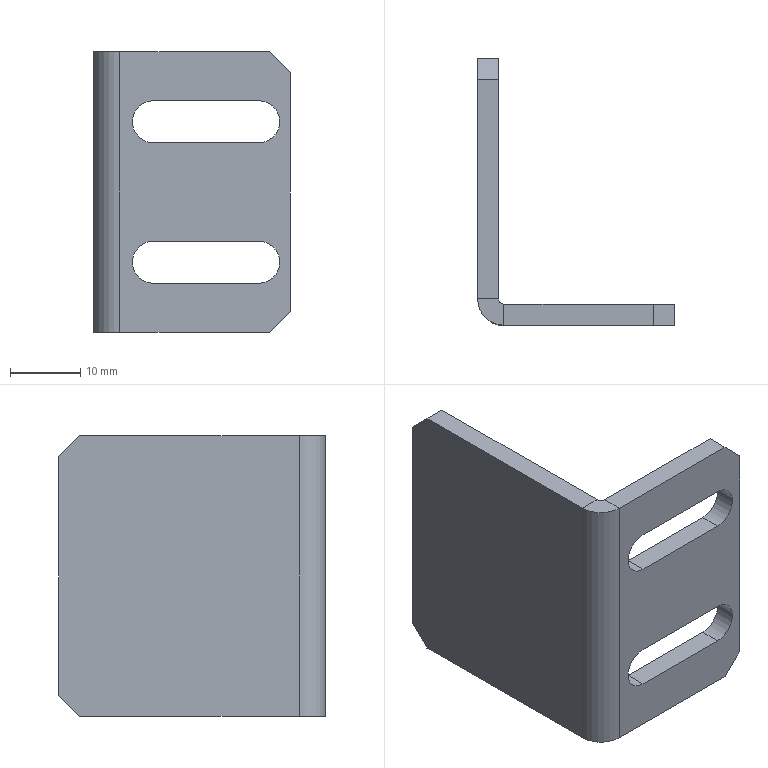Part | STEP file | 11-GYJJ-013-q11 | 1 solid | 26 faces | box 28 x 38 x 40 mm | volume 6681 mm3 | plane 20 | cylinder 6 | commonest cylinder face diameters 6 x4 1.473 x1 7.473 x1
STEP:
#1=CARTESIAN_POINT('',(0.7366,-35.,40.));
#2=VERTEX_POINT('',#1);
#3=CARTESIAN_POINT('',(0.7366,-38.,40.));
#4=VERTEX_POINT('',#3);
#5=CARTESIAN_POINT('',(0.7366,-35.,40.));
#6=DIRECTION('',(0.,-1.,0.));
#7=VECTOR('',#6,1000.);
#8=LINE('',#5,#7);
#9=EDGE_CURVE('',#2,#4,#8,.T.);
#10=ORIENTED_EDGE('',*,*,#9,.F.);
#11=CARTESIAN_POINT('',(0.,-34.263,40.));
#12=VERTEX_POINT('',#11);
#13=CARTESIAN_POINT('',(0.7366,-34.263,40.));
#14=DIRECTION('',(0.,0.,1.));
#15=DIRECTION('',(-1.,0.,0.));
#16=AXIS2_PLACEMENT_3D('',#13,#14,#15);
#17=CIRCLE('',#16,0.7366);
#18=EDGE_CURVE('',#12,#2,#17,.T.);
#19=ORIENTED_EDGE('',*,*,#18,.F.);
#20=CARTESIAN_POINT('',(-3.,-34.263,40.));
#21=VERTEX_POINT('',#20);
#22=CARTESIAN_POINT('',(-3.,-34.263,40.));
#23=DIRECTION('',(1.,0.,0.));
#24=VECTOR('',#23,1000.);
#25=LINE('',#22,#24);
#26=EDGE_CURVE('',#21,#12,#25,.T.);
#27=ORIENTED_EDGE('',*,*,#26,.F.);
#28=CARTESIAN_POINT('',(0.7366,-34.263,40.));
#29=DIRECTION('',(0.,0.,1.));
#30=DIRECTION('',(1.,0.,0.));
#31=AXIS2_PLACEMENT_3D('',#28,#29,#30);
#32=CIRCLE('',#31,3.737);
#33=EDGE_CURVE('',#21,#4,#32,.T.);
#34=ORIENTED_EDGE('',*,*,#33,.T.);
#35=EDGE_LOOP('',(#10,#19,#27,#34));
#36=FACE_OUTER_BOUND('',#35,.T.);
#37=CARTESIAN_POINT('',(0.7366,-35.,40.));
#38=DIRECTION('',(0.,0.,1.));
#39=DIRECTION('',(1.,0.,0.));
#40=AXIS2_PLACEMENT_3D('',#37,#38,#39);
#41=PLANE('',#40);
#42=ADVANCED_FACE('',(#36),#41,.T.);
#43=CARTESIAN_POINT('',(22.,-38.,40.));
#44=VERTEX_POINT('',#43);
#45=CARTESIAN_POINT('',(0.,-38.,40.));
#46=DIRECTION('',(1.,0.,0.));
#47=VECTOR('',#46,1000.);
#48=LINE('',#45,#47);
#49=EDGE_CURVE('',#4,#44,#48,.T.);
#50=ORIENTED_EDGE('',*,*,#49,.T.);
#51=CARTESIAN_POINT('',(22.,-35.,40.));
#52=VERTEX_POINT('',#51);
#53=CARTESIAN_POINT('',(22.,-34.263,40.));
#54=DIRECTION('',(0.,1.,0.));
#55=VECTOR('',#54,1000.);
#56=LINE('',#53,#55);
#57=EDGE_CURVE('',#44,#52,#56,.T.);
#58=ORIENTED_EDGE('',*,*,#57,.T.);
#59=CARTESIAN_POINT('',(0.,-35.,40.));
#60=DIRECTION('',(1.,0.,0.));
#61=VECTOR('',#60,1000.);
#62=LINE('',#59,#61);
#63=EDGE_CURVE('',#2,#52,#62,.T.);
#64=ORIENTED_EDGE('',*,*,#63,.F.);
#65=ORIENTED_EDGE('',*,*,#9,.T.);
#66=EDGE_LOOP('',(#50,#58,#64,#65));
#67=FACE_OUTER_BOUND('',#66,.T.);
#68=CARTESIAN_POINT('',(-3.,-34.263,40.));
#69=DIRECTION('',(0.,0.,1.));
#70=DIRECTION('',(1.,0.,0.));
#71=AXIS2_PLACEMENT_3D('',#68,#69,#70);
#72=PLANE('',#71);
#73=ADVANCED_FACE('',(#67),#72,.T.);
#74=CARTESIAN_POINT('',(0.,-34.263,0.));
#75=VERTEX_POINT('',#74);
#76=CARTESIAN_POINT('',(-3.,-34.263,0.));
#77=VERTEX_POINT('',#76);
#78=CARTESIAN_POINT('',(0.,-34.263,0.));
#79=DIRECTION('',(-1.,0.,0.));
#80=VECTOR('',#79,1000.);
#81=LINE('',#78,#80);
#82=EDGE_CURVE('',#75,#77,#81,.T.);
#83=ORIENTED_EDGE('',*,*,#82,.F.);
#84=CARTESIAN_POINT('',(0.7366,-35.,0.));
#85=VERTEX_POINT('',#84);
#86=CARTESIAN_POINT('',(0.7366,-34.263,0.));
#87=DIRECTION('',(0.,0.,1.));
#88=DIRECTION('',(-1.,0.,0.));
#89=AXIS2_PLACEMENT_3D('',#86,#87,#88);
#90=CIRCLE('',#89,0.7366);
#91=EDGE_CURVE('',#75,#85,#90,.T.);
#92=ORIENTED_EDGE('',*,*,#91,.T.);
#93=CARTESIAN_POINT('',(0.7366,-38.,0.));
#94=VERTEX_POINT('',#93);
#95=CARTESIAN_POINT('',(0.7366,-38.,0.));
#96=DIRECTION('',(0.,1.,0.));
#97=VECTOR('',#96,1000.);
#98=LINE('',#95,#97);
#99=EDGE_CURVE('',#94,#85,#98,.T.);
#100=ORIENTED_EDGE('',*,*,#99,.F.);
#101=CARTESIAN_POINT('',(0.7366,-34.263,0.));
#102=DIRECTION('',(0.,0.,1.));
#103=DIRECTION('',(1.,0.,0.));
#104=AXIS2_PLACEMENT_3D('',#101,#102,#103);
#105=CIRCLE('',#104,3.737);
#106=EDGE_CURVE('',#77,#94,#105,.T.);
#107=ORIENTED_EDGE('',*,*,#106,.F.);
#108=EDGE_LOOP('',(#83,#92,#100,#107));
#109=FACE_OUTER_BOUND('',#108,.T.);
#110=CARTESIAN_POINT('',(0.,-34.263,0.));
#111=DIRECTION('',(0.,0.,-1.));
#112=DIRECTION('',(-1.,0.,0.));
#113=AXIS2_PLACEMENT_3D('',#110,#111,#112);
#114=PLANE('',#113);
#115=ADVANCED_FACE('',(#109),#114,.T.);
#116=CARTESIAN_POINT('',(-3.,-3.,0.));
#117=VERTEX_POINT('',#116);
#118=CARTESIAN_POINT('',(-3.,0.,0.));
#119=DIRECTION('',(0.,-1.,0.));
#120=VECTOR('',#119,1000.);
#121=LINE('',#118,#120);
#122=EDGE_CURVE('',#117,#77,#121,.T.);
#123=ORIENTED_EDGE('',*,*,#122,.F.);
#124=CARTESIAN_POINT('',(0.,-3.,0.));
#125=VERTEX_POINT('',#124);
#126=CARTESIAN_POINT('',(0.7366,-3.,0.));
#127=DIRECTION('',(1.,0.,0.));
#128=VECTOR('',#127,1000.);
#129=LINE('',#126,#128);
#130=EDGE_CURVE('',#117,#125,#129,.T.);
#131=ORIENTED_EDGE('',*,*,#130,.T.);
#132=CARTESIAN_POINT('',(0.,0.,0.));
#133=DIRECTION('',(0.,-1.,0.));
#134=VECTOR('',#133,1000.);
#135=LINE('',#132,#134);
#136=EDGE_CURVE('',#125,#75,#135,.T.);
#137=ORIENTED_EDGE('',*,*,#136,.T.);
#138=ORIENTED_EDGE('',*,*,#82,.T.);
#139=EDGE_LOOP('',(#123,#131,#137,#138));
#140=FACE_OUTER_BOUND('',#139,.T.);
#141=CARTESIAN_POINT('',(0.7366,-38.,0.));
#142=DIRECTION('',(0.,0.,-1.));
#143=DIRECTION('',(-1.,0.,0.));
#144=AXIS2_PLACEMENT_3D('',#141,#142,#143);
#145=PLANE('',#144);
#146=ADVANCED_FACE('',(#140),#145,.T.);
#147=CARTESIAN_POINT('',(20.5,-38.,7.));
#148=VERTEX_POINT('',#147);
#149=CARTESIAN_POINT('',(5.5,-38.,7.));
#150=VERTEX_POINT('',#149);
#151=CARTESIAN_POINT('',(5.5,-38.,7.));
#152=DIRECTION('',(-1.,0.,0.));
#153=VECTOR('',#152,1000.);
#154=LINE('',#151,#153);
#155=EDGE_CURVE('',#148,#150,#154,.T.);
#156=ORIENTED_EDGE('',*,*,#155,.T.);
#157=CARTESIAN_POINT('',(5.5,-38.,13.));
#158=VERTEX_POINT('',#157);
#159=CARTESIAN_POINT('',(5.5,-38.,10.));
#160=DIRECTION('',(0.,1.,0.));
#161=DIRECTION('',(0.,0.,1.));
#162=AXIS2_PLACEMENT_3D('',#159,#160,#161);
#163=CIRCLE('',#162,3.);
#164=EDGE_CURVE('',#150,#158,#163,.T.);
#165=ORIENTED_EDGE('',*,*,#164,.T.);
#166=CARTESIAN_POINT('',(20.5,-38.,13.));
#167=VERTEX_POINT('',#166);
#168=CARTESIAN_POINT('',(5.5,-38.,13.));
#169=DIRECTION('',(1.,0.,0.));
#170=VECTOR('',#169,1000.);
#171=LINE('',#168,#170);
#172=EDGE_CURVE('',#158,#167,#171,.T.);
#173=ORIENTED_EDGE('',*,*,#172,.T.);
#174=CARTESIAN_POINT('',(20.5,-38.,10.));
#175=DIRECTION('',(0.,1.,0.));
#176=DIRECTION('',(0.,0.,1.));
#177=AXIS2_PLACEMENT_3D('',#174,#175,#176);
#178=CIRCLE('',#177,3.);
#179=EDGE_CURVE('',#167,#148,#178,.T.);
#180=ORIENTED_EDGE('',*,*,#179,.T.);
#181=EDGE_LOOP('',(#156,#165,#173,#180));
#182=FACE_BOUND('',#181,.T.);
#183=CARTESIAN_POINT('',(5.5,-38.,33.));
#184=VERTEX_POINT('',#183);
#185=CARTESIAN_POINT('',(20.5,-38.,33.));
#186=VERTEX_POINT('',#185);
#187=CARTESIAN_POINT('',(20.5,-38.,33.));
#188=DIRECTION('',(1.,0.,0.));
#189=VECTOR('',#188,1000.);
#190=LINE('',#187,#189);
#191=EDGE_CURVE('',#184,#186,#190,.T.);
#192=ORIENTED_EDGE('',*,*,#191,.T.);
#193=CARTESIAN_POINT('',(20.5,-38.,27.));
#194=VERTEX_POINT('',#193);
#195=CARTESIAN_POINT('',(20.5,-38.,30.));
#196=DIRECTION('',(0.,1.,0.));
#197=DIRECTION('',(0.,0.,1.));
#198=AXIS2_PLACEMENT_3D('',#195,#196,#197);
#199=CIRCLE('',#198,3.);
#200=EDGE_CURVE('',#186,#194,#199,.T.);
#201=ORIENTED_EDGE('',*,*,#200,.T.);
#202=CARTESIAN_POINT('',(5.5,-38.,27.));
#203=VERTEX_POINT('',#202);
#204=CARTESIAN_POINT('',(20.5,-38.,27.));
#205=DIRECTION('',(-1.,0.,0.));
#206=VECTOR('',#205,1000.);
#207=LINE('',#204,#206);
#208=EDGE_CURVE('',#194,#203,#207,.T.);
#209=ORIENTED_EDGE('',*,*,#208,.T.);
#210=CARTESIAN_POINT('',(5.5,-38.,30.));
#211=DIRECTION('',(0.,1.,0.));
#212=DIRECTION('',(0.,0.,1.));
#213=AXIS2_PLACEMENT_3D('',#210,#211,#212);
#214=CIRCLE('',#213,3.);
#215=EDGE_CURVE('',#203,#184,#214,.T.);
#216=ORIENTED_EDGE('',*,*,#215,.T.);
#217=EDGE_LOOP('',(#192,#201,#209,#216));
#218=FACE_BOUND('',#217,.T.);
#219=CARTESIAN_POINT('',(25.,-38.,37.));
#220=VERTEX_POINT('',#219);
#221=CARTESIAN_POINT('',(25.,-38.,3.));
#222=VERTEX_POINT('',#221);
#223=CARTESIAN_POINT('',(25.,-38.,40.));
#224=DIRECTION('',(0.,0.,-1.));
#225=VECTOR('',#224,1000.);
#226=LINE('',#223,#225);
#227=EDGE_CURVE('',#220,#222,#226,.T.);
#228=ORIENTED_EDGE('',*,*,#227,.F.);
#229=CARTESIAN_POINT('',(25.,-38.,37.));
#230=DIRECTION('',(-0.7071,0.,0.7071));
#231=VECTOR('',#230,1000.);
#232=LINE('',#229,#231);
#233=EDGE_CURVE('',#220,#44,#232,.T.);
#234=ORIENTED_EDGE('',*,*,#233,.T.);
#235=ORIENTED_EDGE('',*,*,#49,.F.);
#236=CARTESIAN_POINT('',(0.7366,-38.,40.));
#237=DIRECTION('',(0.,0.,-1.));
#238=VECTOR('',#237,1000.);
#239=LINE('',#236,#238);
#240=EDGE_CURVE('',#4,#94,#239,.T.);
#241=ORIENTED_EDGE('',*,*,#240,.T.);
#242=CARTESIAN_POINT('',(22.,-38.,0.));
#243=VERTEX_POINT('',#242);
#244=CARTESIAN_POINT('',(0.,-38.,0.));
#245=DIRECTION('',(1.,0.,0.));
#246=VECTOR('',#245,1000.);
#247=LINE('',#244,#246);
#248=EDGE_CURVE('',#94,#243,#247,.T.);
#249=ORIENTED_EDGE('',*,*,#248,.T.);
#250=CARTESIAN_POINT('',(22.,-38.,0.));
#251=DIRECTION('',(0.7071,0.,0.7071));
#252=VECTOR('',#251,1000.);
#253=LINE('',#250,#252);
#254=EDGE_CURVE('',#243,#222,#253,.T.);
#255=ORIENTED_EDGE('',*,*,#254,.T.);
#256=EDGE_LOOP('',(#228,#234,#235,#241,#249,#255));
#257=FACE_OUTER_BOUND('',#256,.T.);
#258=CARTESIAN_POINT('',(0.,-38.,40.));
#259=DIRECTION('',(0.,1.,0.));
#260=DIRECTION('',(0.,0.,1.));
#261=AXIS2_PLACEMENT_3D('',#258,#259,#260);
#262=PLANE('',#261);
#263=ADVANCED_FACE('',(#182,#218,#257),#262,.F.);
#264=CARTESIAN_POINT('',(25.,-35.,37.));
#265=VERTEX_POINT('',#264);
#266=CARTESIAN_POINT('',(25.,-35.,3.));
#267=VERTEX_POINT('',#266);
#268=CARTESIAN_POINT('',(25.,-35.,40.));
#269=DIRECTION('',(0.,0.,-1.));
#270=VECTOR('',#269,1000.);
#271=LINE('',#268,#270);
#272=EDGE_CURVE('',#265,#267,#271,.T.);
#273=ORIENTED_EDGE('',*,*,#272,.F.);
#274=CARTESIAN_POINT('',(25.,-35.,37.));
#275=DIRECTION('',(0.,-1.,0.));
#276=VECTOR('',#275,1000.);
#277=LINE('',#274,#276);
#278=EDGE_CURVE('',#265,#220,#277,.T.);
#279=ORIENTED_EDGE('',*,*,#278,.T.);
#280=ORIENTED_EDGE('',*,*,#227,.T.);
#281=CARTESIAN_POINT('',(25.,-35.,3.));
#282=DIRECTION('',(0.,1.,0.));
#283=VECTOR('',#282,1000.);
#284=LINE('',#281,#283);
#285=EDGE_CURVE('',#222,#267,#284,.T.);
#286=ORIENTED_EDGE('',*,*,#285,.T.);
#287=EDGE_LOOP('',(#273,#279,#280,#286));
#288=FACE_OUTER_BOUND('',#287,.T.);
#289=CARTESIAN_POINT('',(25.,-35.,40.));
#290=DIRECTION('',(1.,0.,0.));
#291=DIRECTION('',(0.,0.,-1.));
#292=AXIS2_PLACEMENT_3D('',#289,#290,#291);
#293=PLANE('',#292);
#294=ADVANCED_FACE('',(#288),#293,.T.);
#295=CARTESIAN_POINT('',(5.5,-35.,7.));
#296=VERTEX_POINT('',#295);
#297=CARTESIAN_POINT('',(5.5,-35.,13.));
#298=VERTEX_POINT('',#297);
#299=CARTESIAN_POINT('',(5.5,-35.,10.));
#300=DIRECTION('',(0.,1.,0.));
#301=DIRECTION('',(0.,0.,1.));
#302=AXIS2_PLACEMENT_3D('',#299,#300,#301);
#303=CIRCLE('',#302,3.);
#304=EDGE_CURVE('',#296,#298,#303,.T.);
#305=ORIENTED_EDGE('',*,*,#304,.F.);
#306=CARTESIAN_POINT('',(20.5,-35.,7.));
#307=VERTEX_POINT('',#306);
#308=CARTESIAN_POINT('',(5.5,-35.,7.));
#309=DIRECTION('',(-1.,0.,0.));
#310=VECTOR('',#309,1000.);
#311=LINE('',#308,#310);
#312=EDGE_CURVE('',#307,#296,#311,.T.);
#313=ORIENTED_EDGE('',*,*,#312,.F.);
#314=CARTESIAN_POINT('',(20.5,-35.,13.));
#315=VERTEX_POINT('',#314);
#316=CARTESIAN_POINT('',(20.5,-35.,10.));
#317=DIRECTION('',(0.,1.,0.));
#318=DIRECTION('',(0.,0.,1.));
#319=AXIS2_PLACEMENT_3D('',#316,#317,#318);
#320=CIRCLE('',#319,3.);
#321=EDGE_CURVE('',#315,#307,#320,.T.);
#322=ORIENTED_EDGE('',*,*,#321,.F.);
#323=CARTESIAN_POINT('',(5.5,-35.,13.));
#324=DIRECTION('',(1.,0.,0.));
#325=VECTOR('',#324,1000.);
#326=LINE('',#323,#325);
#327=EDGE_CURVE('',#298,#315,#326,.T.);
#328=ORIENTED_EDGE('',*,*,#327,.F.);
#329=EDGE_LOOP('',(#305,#313,#322,#328));
#330=FACE_BOUND('',#329,.T.);
#331=CARTESIAN_POINT('',(20.5,-35.,33.));
#332=VERTEX_POINT('',#331);
#333=CARTESIAN_POINT('',(20.5,-35.,27.));
#334=VERTEX_POINT('',#333);
#335=CARTESIAN_POINT('',(20.5,-35.,30.));
#336=DIRECTION('',(0.,1.,0.));
#337=DIRECTION('',(0.,0.,1.));
#338=AXIS2_PLACEMENT_3D('',#335,#336,#337);
#339=CIRCLE('',#338,3.);
#340=EDGE_CURVE('',#332,#334,#339,.T.);
#341=ORIENTED_EDGE('',*,*,#340,.F.);
#342=CARTESIAN_POINT('',(5.5,-35.,33.));
#343=VERTEX_POINT('',#342);
#344=CARTESIAN_POINT('',(20.5,-35.,33.));
#345=DIRECTION('',(1.,0.,0.));
#346=VECTOR('',#345,1000.);
#347=LINE('',#344,#346);
#348=EDGE_CURVE('',#343,#332,#347,.T.);
#349=ORIENTED_EDGE('',*,*,#348,.F.);
#350=CARTESIAN_POINT('',(5.5,-35.,27.));
#351=VERTEX_POINT('',#350);
#352=CARTESIAN_POINT('',(5.5,-35.,30.));
#353=DIRECTION('',(0.,1.,0.));
#354=DIRECTION('',(0.,0.,1.));
#355=AXIS2_PLACEMENT_3D('',#352,#353,#354);
#356=CIRCLE('',#355,3.);
#357=EDGE_CURVE('',#351,#343,#356,.T.);
#358=ORIENTED_EDGE('',*,*,#357,.F.);
#359=CARTESIAN_POINT('',(20.5,-35.,27.));
#360=DIRECTION('',(-1.,0.,0.));
#361=VECTOR('',#360,1000.);
#362=LINE('',#359,#361);
#363=EDGE_CURVE('',#334,#351,#362,.T.);
#364=ORIENTED_EDGE('',*,*,#363,.F.);
#365=EDGE_LOOP('',(#341,#349,#358,#364));
#366=FACE_BOUND('',#365,.T.);
#367=ORIENTED_EDGE('',*,*,#63,.T.);
#368=CARTESIAN_POINT('',(11.,-35.,51.));
#369=DIRECTION('',(0.7071,0.,-0.7071));
#370=VECTOR('',#369,1000.);
#371=LINE('',#368,#370);
#372=EDGE_CURVE('',#52,#265,#371,.T.);
#373=ORIENTED_EDGE('',*,*,#372,.T.);
#374=ORIENTED_EDGE('',*,*,#272,.T.);
#375=CARTESIAN_POINT('',(22.,-35.,0.));
#376=VERTEX_POINT('',#375);
#377=CARTESIAN_POINT('',(31.,-35.,9.));
#378=DIRECTION('',(-0.7071,0.,-0.7071));
#379=VECTOR('',#378,1000.);
#380=LINE('',#377,#379);
#381=EDGE_CURVE('',#267,#376,#380,.T.);
#382=ORIENTED_EDGE('',*,*,#381,.T.);
#383=CARTESIAN_POINT('',(0.,-35.,0.));
#384=DIRECTION('',(1.,0.,0.));
#385=VECTOR('',#384,1000.);
#386=LINE('',#383,#385);
#387=EDGE_CURVE('',#85,#376,#386,.T.);
#388=ORIENTED_EDGE('',*,*,#387,.F.);
#389=CARTESIAN_POINT('',(0.7366,-35.,40.));
#390=DIRECTION('',(0.,0.,-1.));
#391=VECTOR('',#390,1000.);
#392=LINE('',#389,#391);
#393=EDGE_CURVE('',#2,#85,#392,.T.);
#394=ORIENTED_EDGE('',*,*,#393,.F.);
#395=EDGE_LOOP('',(#367,#373,#374,#382,#388,#394));
#396=FACE_OUTER_BOUND('',#395,.T.);
#397=CARTESIAN_POINT('',(0.,-35.,40.));
#398=DIRECTION('',(0.,1.,0.));
#399=DIRECTION('',(0.,0.,1.));
#400=AXIS2_PLACEMENT_3D('',#397,#398,#399);
#401=PLANE('',#400);
#402=ADVANCED_FACE('',(#330,#366,#396),#401,.T.);
#403=ORIENTED_EDGE('',*,*,#91,.F.);
#404=CARTESIAN_POINT('',(0.,-34.263,40.));
#405=DIRECTION('',(0.,0.,-1.));
#406=VECTOR('',#405,1000.);
#407=LINE('',#404,#406);
#408=EDGE_CURVE('',#12,#75,#407,.T.);
#409=ORIENTED_EDGE('',*,*,#408,.F.);
#410=ORIENTED_EDGE('',*,*,#18,.T.);
#411=ORIENTED_EDGE('',*,*,#393,.T.);
#412=EDGE_LOOP('',(#403,#409,#410,#411));
#413=FACE_OUTER_BOUND('',#412,.T.);
#414=CARTESIAN_POINT('',(0.7366,-34.263,40.));
#415=DIRECTION('',(0.,0.,-1.));
#416=DIRECTION('',(-1.,0.,0.));
#417=AXIS2_PLACEMENT_3D('',#414,#415,#416);
#418=CYLINDRICAL_SURFACE('',#417,0.7366);
#419=ADVANCED_FACE('',(#413),#418,.F.);
#420=CARTESIAN_POINT('',(0.,0.,37.));
#421=VERTEX_POINT('',#420);
#422=CARTESIAN_POINT('',(0.,0.,3.));
#423=VERTEX_POINT('',#422);
#424=CARTESIAN_POINT('',(0.,0.,40.));
#425=DIRECTION('',(0.,0.,-1.));
#426=VECTOR('',#425,1000.);
#427=LINE('',#424,#426);
#428=EDGE_CURVE('',#421,#423,#427,.T.);
#429=ORIENTED_EDGE('',*,*,#428,.F.);
#430=CARTESIAN_POINT('',(0.,-3.,40.));
#431=VERTEX_POINT('',#430);
#432=CARTESIAN_POINT('',(0.,-1.5,38.5));
#433=DIRECTION('',(0.,-0.7071,0.7071));
#434=VECTOR('',#433,1000.);
#435=LINE('',#432,#434);
#436=EDGE_CURVE('',#421,#431,#435,.T.);
#437=ORIENTED_EDGE('',*,*,#436,.T.);
#438=CARTESIAN_POINT('',(0.,0.,40.));
#439=DIRECTION('',(0.,-1.,0.));
#440=VECTOR('',#439,1000.);
#441=LINE('',#438,#440);
#442=EDGE_CURVE('',#431,#12,#441,.T.);
#443=ORIENTED_EDGE('',*,*,#442,.T.);
#444=ORIENTED_EDGE('',*,*,#408,.T.);
#445=ORIENTED_EDGE('',*,*,#136,.F.);
#446=CARTESIAN_POINT('',(0.,18.5,21.5));
#447=DIRECTION('',(0.,0.7071,0.7071));
#448=VECTOR('',#447,1000.);
#449=LINE('',#446,#448);
#450=EDGE_CURVE('',#125,#423,#449,.T.);
#451=ORIENTED_EDGE('',*,*,#450,.T.);
#452=EDGE_LOOP('',(#429,#437,#443,#444,#445,#451));
#453=FACE_OUTER_BOUND('',#452,.T.);
#454=CARTESIAN_POINT('',(0.,0.,40.));
#455=DIRECTION('',(1.,0.,0.));
#456=DIRECTION('',(0.,1.,0.));
#457=AXIS2_PLACEMENT_3D('',#454,#455,#456);
#458=PLANE('',#457);
#459=ADVANCED_FACE('',(#453),#458,.T.);
#460=CARTESIAN_POINT('',(-3.,0.,37.));
#461=VERTEX_POINT('',#460);
#462=CARTESIAN_POINT('',(-3.,0.,3.));
#463=VERTEX_POINT('',#462);
#464=CARTESIAN_POINT('',(-3.,0.,40.));
#465=DIRECTION('',(0.,0.,-1.));
#466=VECTOR('',#465,1000.);
#467=LINE('',#464,#466);
#468=EDGE_CURVE('',#461,#463,#467,.T.);
#469=ORIENTED_EDGE('',*,*,#468,.F.);
#470=CARTESIAN_POINT('',(0.,0.,37.));
#471=DIRECTION('',(1.,0.,0.));
#472=VECTOR('',#471,1000.);
#473=LINE('',#470,#472);
#474=EDGE_CURVE('',#461,#421,#473,.T.);
#475=ORIENTED_EDGE('',*,*,#474,.T.);
#476=ORIENTED_EDGE('',*,*,#428,.T.);
#477=CARTESIAN_POINT('',(-3.,0.,3.));
#478=DIRECTION('',(-1.,0.,0.));
#479=VECTOR('',#478,1000.);
#480=LINE('',#477,#479);
#481=EDGE_CURVE('',#423,#463,#480,.T.);
#482=ORIENTED_EDGE('',*,*,#481,.T.);
#483=EDGE_LOOP('',(#469,#475,#476,#482));
#484=FACE_OUTER_BOUND('',#483,.T.);
#485=CARTESIAN_POINT('',(-3.,0.,40.));
#486=DIRECTION('',(0.,1.,0.));
#487=DIRECTION('',(-1.,0.,0.));
#488=AXIS2_PLACEMENT_3D('',#485,#486,#487);
#489=PLANE('',#488);
#490=ADVANCED_FACE('',(#484),#489,.T.);
#491=CARTESIAN_POINT('',(-3.,-3.,40.));
#492=VERTEX_POINT('',#491);
#493=CARTESIAN_POINT('',(-3.,0.,40.));
#494=DIRECTION('',(0.,-1.,0.));
#495=VECTOR('',#494,1000.);
#496=LINE('',#493,#495);
#497=EDGE_CURVE('',#492,#21,#496,.T.);
#498=ORIENTED_EDGE('',*,*,#497,.F.);
#499=CARTESIAN_POINT('',(-3.,0.,37.));
#500=DIRECTION('',(0.,0.7071,-0.7071));
#501=VECTOR('',#500,1000.);
#502=LINE('',#499,#501);
#503=EDGE_CURVE('',#492,#461,#502,.T.);
#504=ORIENTED_EDGE('',*,*,#503,.T.);
#505=ORIENTED_EDGE('',*,*,#468,.T.);
#506=CARTESIAN_POINT('',(-3.,-3.,0.));
#507=DIRECTION('',(0.,-0.7071,-0.7071));
#508=VECTOR('',#507,1000.);
#509=LINE('',#506,#508);
#510=EDGE_CURVE('',#463,#117,#509,.T.);
#511=ORIENTED_EDGE('',*,*,#510,.T.);
#512=ORIENTED_EDGE('',*,*,#122,.T.);
#513=CARTESIAN_POINT('',(-3.,-34.263,40.));
#514=DIRECTION('',(0.,0.,-1.));
#515=VECTOR('',#514,1000.);
#516=LINE('',#513,#515);
#517=EDGE_CURVE('',#21,#77,#516,.T.);
#518=ORIENTED_EDGE('',*,*,#517,.F.);
#519=EDGE_LOOP('',(#498,#504,#505,#511,#512,#518));
#520=FACE_OUTER_BOUND('',#519,.T.);
#521=CARTESIAN_POINT('',(-3.,0.,40.));
#522=DIRECTION('',(1.,0.,0.));
#523=DIRECTION('',(0.,1.,0.));
#524=AXIS2_PLACEMENT_3D('',#521,#522,#523);
#525=PLANE('',#524);
#526=ADVANCED_FACE('',(#520),#525,.F.);
#527=ORIENTED_EDGE('',*,*,#106,.T.);
#528=ORIENTED_EDGE('',*,*,#240,.F.);
#529=ORIENTED_EDGE('',*,*,#33,.F.);
#530=ORIENTED_EDGE('',*,*,#517,.T.);
#531=EDGE_LOOP('',(#527,#528,#529,#530));
#532=FACE_OUTER_BOUND('',#531,.T.);
#533=CARTESIAN_POINT('',(0.7366,-34.263,40.));
#534=DIRECTION('',(0.,0.,-1.));
#535=DIRECTION('',(-1.,0.,0.));
#536=AXIS2_PLACEMENT_3D('',#533,#534,#535);
#537=CYLINDRICAL_SURFACE('',#536,3.737);
#538=ADVANCED_FACE('',(#532),#537,.T.);
#539=ORIENTED_EDGE('',*,*,#442,.F.);
#540=CARTESIAN_POINT('',(-3.,-3.,40.));
#541=DIRECTION('',(-1.,0.,0.));
#542=VECTOR('',#541,1000.);
#543=LINE('',#540,#542);
#544=EDGE_CURVE('',#431,#492,#543,.T.);
#545=ORIENTED_EDGE('',*,*,#544,.T.);
#546=ORIENTED_EDGE('',*,*,#497,.T.);
#547=ORIENTED_EDGE('',*,*,#26,.T.);
#548=EDGE_LOOP('',(#539,#545,#546,#547));
#549=FACE_OUTER_BOUND('',#548,.T.);
#550=CARTESIAN_POINT('',(0.7366,-34.263,40.));
#551=DIRECTION('',(0.,0.,-1.));
#552=DIRECTION('',(-1.,0.,0.));
#553=AXIS2_PLACEMENT_3D('',#550,#551,#552);
#554=PLANE('',#553);
#555=ADVANCED_FACE('',(#549),#554,.F.);
#556=ORIENTED_EDGE('',*,*,#387,.T.);
#557=CARTESIAN_POINT('',(22.,-34.263,0.));
#558=DIRECTION('',(0.,-1.,0.));
#559=VECTOR('',#558,1000.);
#560=LINE('',#557,#559);
#561=EDGE_CURVE('',#376,#243,#560,.T.);
#562=ORIENTED_EDGE('',*,*,#561,.T.);
#563=ORIENTED_EDGE('',*,*,#248,.F.);
#564=ORIENTED_EDGE('',*,*,#99,.T.);
#565=EDGE_LOOP('',(#556,#562,#563,#564));
#566=FACE_OUTER_BOUND('',#565,.T.);
#567=CARTESIAN_POINT('',(0.7366,-34.263,0.));
#568=DIRECTION('',(0.,0.,-1.));
#569=DIRECTION('',(-1.,0.,0.));
#570=AXIS2_PLACEMENT_3D('',#567,#568,#569);
#571=PLANE('',#570);
#572=ADVANCED_FACE('',(#566),#571,.T.);
#573=ORIENTED_EDGE('',*,*,#372,.F.);
#574=ORIENTED_EDGE('',*,*,#57,.F.);
#575=ORIENTED_EDGE('',*,*,#233,.F.);
#576=ORIENTED_EDGE('',*,*,#278,.F.);
#577=EDGE_LOOP('',(#573,#574,#575,#576));
#578=FACE_OUTER_BOUND('',#577,.T.);
#579=CARTESIAN_POINT('',(25.,-35.,37.));
#580=DIRECTION('',(-0.7071,0.,-0.7071));
#581=DIRECTION('',(0.,-1.,0.));
#582=AXIS2_PLACEMENT_3D('',#579,#580,#581);
#583=PLANE('',#582);
#584=ADVANCED_FACE('',(#578),#583,.F.);
#585=ORIENTED_EDGE('',*,*,#381,.F.);
#586=ORIENTED_EDGE('',*,*,#285,.F.);
#587=ORIENTED_EDGE('',*,*,#254,.F.);
#588=ORIENTED_EDGE('',*,*,#561,.F.);
#589=EDGE_LOOP('',(#585,#586,#587,#588));
#590=FACE_OUTER_BOUND('',#589,.T.);
#591=CARTESIAN_POINT('',(22.,-34.263,0.));
#592=DIRECTION('',(-0.7071,0.,0.7071));
#593=DIRECTION('',(0.,-1.,0.));
#594=AXIS2_PLACEMENT_3D('',#591,#592,#593);
#595=PLANE('',#594);
#596=ADVANCED_FACE('',(#590),#595,.F.);
#597=ORIENTED_EDGE('',*,*,#503,.F.);
#598=ORIENTED_EDGE('',*,*,#544,.F.);
#599=ORIENTED_EDGE('',*,*,#436,.F.);
#600=ORIENTED_EDGE('',*,*,#474,.F.);
#601=EDGE_LOOP('',(#597,#598,#599,#600));
#602=FACE_OUTER_BOUND('',#601,.T.);
#603=CARTESIAN_POINT('',(-3.,0.,37.));
#604=DIRECTION('',(0.,0.7071,0.7071));
#605=DIRECTION('',(-1.,0.,0.));
#606=AXIS2_PLACEMENT_3D('',#603,#604,#605);
#607=PLANE('',#606);
#608=ADVANCED_FACE('',(#602),#607,.T.);
#609=ORIENTED_EDGE('',*,*,#510,.F.);
#610=ORIENTED_EDGE('',*,*,#481,.F.);
#611=ORIENTED_EDGE('',*,*,#450,.F.);
#612=ORIENTED_EDGE('',*,*,#130,.F.);
#613=EDGE_LOOP('',(#609,#610,#611,#612));
#614=FACE_OUTER_BOUND('',#613,.T.);
#615=CARTESIAN_POINT('',(0.7366,-3.,0.));
#616=DIRECTION('',(0.,-0.7071,0.7071));
#617=DIRECTION('',(1.,0.,0.));
#618=AXIS2_PLACEMENT_3D('',#615,#616,#617);
#619=PLANE('',#618);
#620=ADVANCED_FACE('',(#614),#619,.F.);
#621=ORIENTED_EDGE('',*,*,#340,.T.);
#622=CARTESIAN_POINT('',(20.5,-38.,27.));
#623=DIRECTION('',(0.,1.,0.));
#624=VECTOR('',#623,1000.);
#625=LINE('',#622,#624);
#626=EDGE_CURVE('',#194,#334,#625,.T.);
#627=ORIENTED_EDGE('',*,*,#626,.F.);
#628=ORIENTED_EDGE('',*,*,#200,.F.);
#629=CARTESIAN_POINT('',(20.5,-38.,33.));
#630=DIRECTION('',(0.,1.,0.));
#631=VECTOR('',#630,1000.);
#632=LINE('',#629,#631);
#633=EDGE_CURVE('',#186,#332,#632,.T.);
#634=ORIENTED_EDGE('',*,*,#633,.T.);
#635=EDGE_LOOP('',(#621,#627,#628,#634));
#636=FACE_OUTER_BOUND('',#635,.T.);
#637=CARTESIAN_POINT('',(20.5,-38.,30.));
#638=DIRECTION('',(0.,1.,0.));
#639=DIRECTION('',(0.,0.,1.));
#640=AXIS2_PLACEMENT_3D('',#637,#638,#639);
#641=CYLINDRICAL_SURFACE('',#640,3.);
#642=ADVANCED_FACE('',(#636),#641,.F.);
#643=ORIENTED_EDGE('',*,*,#348,.T.);
#644=ORIENTED_EDGE('',*,*,#633,.F.);
#645=ORIENTED_EDGE('',*,*,#191,.F.);
#646=CARTESIAN_POINT('',(5.5,-38.,33.));
#647=DIRECTION('',(0.,1.,0.));
#648=VECTOR('',#647,1000.);
#649=LINE('',#646,#648);
#650=EDGE_CURVE('',#184,#343,#649,.T.);
#651=ORIENTED_EDGE('',*,*,#650,.T.);
#652=EDGE_LOOP('',(#643,#644,#645,#651));
#653=FACE_OUTER_BOUND('',#652,.T.);
#654=CARTESIAN_POINT('',(20.5,-38.,33.));
#655=DIRECTION('',(0.,0.,1.));
#656=DIRECTION('',(1.,0.,0.));
#657=AXIS2_PLACEMENT_3D('',#654,#655,#656);
#658=PLANE('',#657);
#659=ADVANCED_FACE('',(#653),#658,.F.);
#660=ORIENTED_EDGE('',*,*,#357,.T.);
#661=ORIENTED_EDGE('',*,*,#650,.F.);
#662=ORIENTED_EDGE('',*,*,#215,.F.);
#663=CARTESIAN_POINT('',(5.5,-38.,27.));
#664=DIRECTION('',(0.,1.,0.));
#665=VECTOR('',#664,1000.);
#666=LINE('',#663,#665);
#667=EDGE_CURVE('',#203,#351,#666,.T.);
#668=ORIENTED_EDGE('',*,*,#667,.T.);
#669=EDGE_LOOP('',(#660,#661,#662,#668));
#670=FACE_OUTER_BOUND('',#669,.T.);
#671=CARTESIAN_POINT('',(5.5,-38.,30.));
#672=DIRECTION('',(0.,1.,0.));
#673=DIRECTION('',(0.,0.,1.));
#674=AXIS2_PLACEMENT_3D('',#671,#672,#673);
#675=CYLINDRICAL_SURFACE('',#674,3.);
#676=ADVANCED_FACE('',(#670),#675,.F.);
#677=ORIENTED_EDGE('',*,*,#363,.T.);
#678=ORIENTED_EDGE('',*,*,#667,.F.);
#679=ORIENTED_EDGE('',*,*,#208,.F.);
#680=ORIENTED_EDGE('',*,*,#626,.T.);
#681=EDGE_LOOP('',(#677,#678,#679,#680));
#682=FACE_OUTER_BOUND('',#681,.T.);
#683=CARTESIAN_POINT('',(20.5,-38.,27.));
#684=DIRECTION('',(0.,0.,-1.));
#685=DIRECTION('',(-1.,0.,0.));
#686=AXIS2_PLACEMENT_3D('',#683,#684,#685);
#687=PLANE('',#686);
#688=ADVANCED_FACE('',(#682),#687,.F.);
#689=ORIENTED_EDGE('',*,*,#304,.T.);
#690=CARTESIAN_POINT('',(5.5,-38.,13.));
#691=DIRECTION('',(0.,1.,0.));
#692=VECTOR('',#691,1000.);
#693=LINE('',#690,#692);
#694=EDGE_CURVE('',#158,#298,#693,.T.);
#695=ORIENTED_EDGE('',*,*,#694,.F.);
#696=ORIENTED_EDGE('',*,*,#164,.F.);
#697=CARTESIAN_POINT('',(5.5,-38.,7.));
#698=DIRECTION('',(0.,1.,0.));
#699=VECTOR('',#698,1000.);
#700=LINE('',#697,#699);
#701=EDGE_CURVE('',#150,#296,#700,.T.);
#702=ORIENTED_EDGE('',*,*,#701,.T.);
#703=EDGE_LOOP('',(#689,#695,#696,#702));
#704=FACE_OUTER_BOUND('',#703,.T.);
#705=CARTESIAN_POINT('',(5.5,-38.,10.));
#706=DIRECTION('',(0.,1.,0.));
#707=DIRECTION('',(0.,0.,1.));
#708=AXIS2_PLACEMENT_3D('',#705,#706,#707);
#709=CYLINDRICAL_SURFACE('',#708,3.);
#710=ADVANCED_FACE('',(#704),#709,.F.);
#711=ORIENTED_EDGE('',*,*,#312,.T.);
#712=ORIENTED_EDGE('',*,*,#701,.F.);
#713=ORIENTED_EDGE('',*,*,#155,.F.);
#714=CARTESIAN_POINT('',(20.5,-38.,7.));
#715=DIRECTION('',(0.,1.,0.));
#716=VECTOR('',#715,1000.);
#717=LINE('',#714,#716);
#718=EDGE_CURVE('',#148,#307,#717,.T.);
#719=ORIENTED_EDGE('',*,*,#718,.T.);
#720=EDGE_LOOP('',(#711,#712,#713,#719));
#721=FACE_OUTER_BOUND('',#720,.T.);
#722=CARTESIAN_POINT('',(5.5,-38.,7.));
#723=DIRECTION('',(0.,0.,-1.));
#724=DIRECTION('',(-1.,0.,0.));
#725=AXIS2_PLACEMENT_3D('',#722,#723,#724);
#726=PLANE('',#725);
#727=ADVANCED_FACE('',(#721),#726,.F.);
#728=ORIENTED_EDGE('',*,*,#321,.T.);
#729=ORIENTED_EDGE('',*,*,#718,.F.);
#730=ORIENTED_EDGE('',*,*,#179,.F.);
#731=CARTESIAN_POINT('',(20.5,-38.,13.));
#732=DIRECTION('',(0.,1.,0.));
#733=VECTOR('',#732,1000.);
#734=LINE('',#731,#733);
#735=EDGE_CURVE('',#167,#315,#734,.T.);
#736=ORIENTED_EDGE('',*,*,#735,.T.);
#737=EDGE_LOOP('',(#728,#729,#730,#736));
#738=FACE_OUTER_BOUND('',#737,.T.);
#739=CARTESIAN_POINT('',(20.5,-38.,10.));
#740=DIRECTION('',(0.,1.,0.));
#741=DIRECTION('',(0.,0.,1.));
#742=AXIS2_PLACEMENT_3D('',#739,#740,#741);
#743=CYLINDRICAL_SURFACE('',#742,3.);
#744=ADVANCED_FACE('',(#738),#743,.F.);
#745=ORIENTED_EDGE('',*,*,#327,.T.);
#746=ORIENTED_EDGE('',*,*,#735,.F.);
#747=ORIENTED_EDGE('',*,*,#172,.F.);
#748=ORIENTED_EDGE('',*,*,#694,.T.);
#749=EDGE_LOOP('',(#745,#746,#747,#748));
#750=FACE_OUTER_BOUND('',#749,.T.);
#751=CARTESIAN_POINT('',(5.5,-38.,13.));
#752=DIRECTION('',(0.,0.,1.));
#753=DIRECTION('',(1.,0.,0.));
#754=AXIS2_PLACEMENT_3D('',#751,#752,#753);
#755=PLANE('',#754);
#756=ADVANCED_FACE('',(#750),#755,.F.);
#757=CLOSED_SHELL('',(#42,#73,#115,#146,#263,#294,#402,#419,#459,#490,#526,#538,#555,#572,#584,#596,#608,#620,#642,#659,#676,#688,#710,#727,#744,#756));
#758=MANIFOLD_SOLID_BREP('',#757);
#759=CARTESIAN_POINT('',(0.,0.,0.));
#760=DIRECTION('',(0.,0.,1.));
#761=DIRECTION('',(1.,0.,0.));
#762=AXIS2_PLACEMENT_3D('',#759,#760,#761);
#763=(LENGTH_UNIT()NAMED_UNIT(*)SI_UNIT(.MILLI.,.METRE.));
#764=UNCERTAINTY_MEASURE_WITH_UNIT(LENGTH_MEASURE(0.00001),#763,'','');
#765=(NAMED_UNIT(*)PLANE_ANGLE_UNIT()SI_UNIT($,.RADIAN.));
#766=(NAMED_UNIT(*)SI_UNIT($,.STERADIAN.)SOLID_ANGLE_UNIT());
#767=(GEOMETRIC_REPRESENTATION_CONTEXT(3)GLOBAL_UNCERTAINTY_ASSIGNED_CONTEXT((#764))GLOBAL_UNIT_ASSIGNED_CONTEXT((#763,#765,#766))REPRESENTATION_CONTEXT('',''));
#768=ADVANCED_BREP_SHAPE_REPRESENTATION('',(#758,#762),#767);